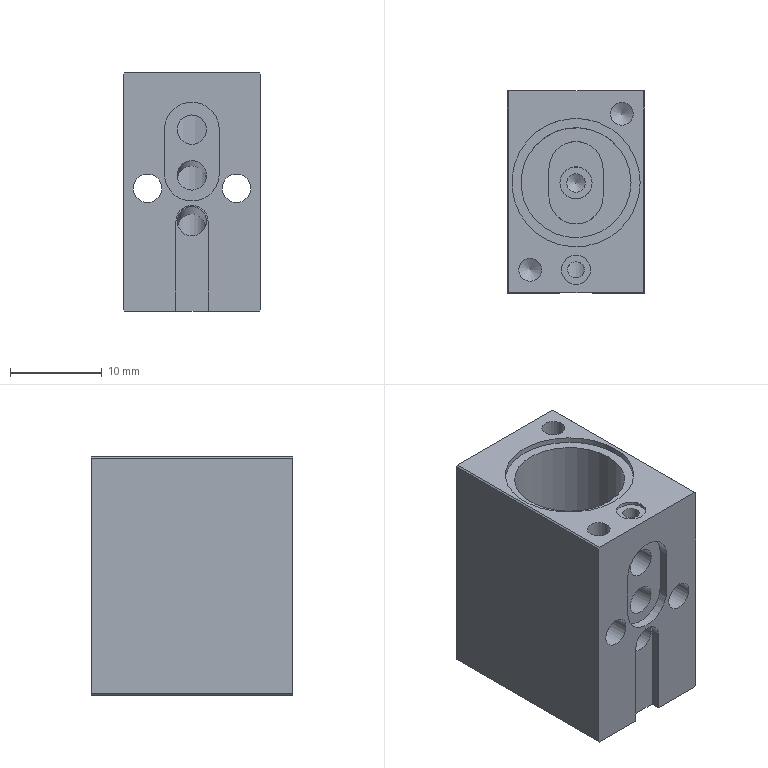NC program | NX | posted with a generic post | part box 15 x 22 x 26 mm
Lines 1 to 1765 of 5185, first 1455 of 1737 lines:
N10 G17 G21 G94 G90
(DRILLING_2 , TOOL : D4点钻)
N12 T02 M6
N14 G54
N16 G17 G0 G90 X0. Y12. B0. C0. S3000 M3
N18 G43 Z30. H2
N20 G94 G81 G98 Z-1.25 F200. R3.
N22 X5. Y19.5
N24 X0. Y2.5
N26 X-5.
N28 G80
N30 G0 X-5. Y2.5 Z30.
N32 M5
(DRILLING_2_COPY_2 , TOOL : D1.8钻头)
N34 T07 M6
N36 G54
N38 G17 G0 G90 X0. Y2.5 B0. C0. S3000 M3
N40 G43 Z30. H7
N42 G94 G81 G98 Z-6.5 F200. R3.
N44 G80
N46 G0 X0. Y2.5 Z30.
N48 M5
(DRILLING_2_COPY_1 , TOOL : D2.3钻头)
N50 T08 M6
N52 G54
N54 G17 G0 G90 X5. Y19.5 B0. C0. S3000 M3
N56 G43 Z30. H8
N58 G94 G81 G98 Z-8. F200. R3.
N60 X-5. Y2.5
N62 G80
N64 G0 X-5. Y2.5 Z30.
N66 M5
(DRILLING_2_COPY , TOOL : Z5.5)
N68 T09 M6
N70 G54
N72 G17 G0 G90 X0. Y12. B0. C0. S3000 M3
N74 G43 Z30. H9
N76 G94 G81 G99 Z-14. F200. R3.
N78 G80
N80 G0 X0. Y12. Z30.
N82 M5
(PLANAR_MILL_6 , TOOL : D8开粗)
N84 T13 M6
N86 G54
N88 G17 G0 G90 X-1.873 Y12.414 B0. C0. S4500 M3
N90 G43 Z30. H13
N92 Z1.
N94 G94 G1 X-1.9 Y11.661 Z0.987 F1000.
N96 X-1.671 Y11.035 Z0.975
N98 X-1.244 Y10.524 Z0.964
N100 X-0.656 Y10.185 Z0.952
N102 X0.17 Y10.078 Z0.937
N104 X0.965 Y10.329 Z0.923
N106 X1.58 Y10.891 Z0.908
N108 X1.9 Y11.661 Z0.893
N110 Y12.339 Z0.882
N112 X1.58 Y13.109 Z0.867
N114 X0.965 Y13.671 Z0.853
N116 X0.17 Y13.922 Z0.838
N118 X-0.656 Y13.815 Z0.823
N120 X-1.244 Y13.476 Z0.812
N122 X-1.671 Y12.965 Z0.8
N124 X-1.9 Y12.339 Z0.788
N126 Y11.661 Z0.777
N128 X-1.671 Y11.035 Z0.765
N130 X-1.244 Y10.524 Z0.753
N132 X-0.656 Y10.185 Z0.741
N134 X0.17 Y10.078 Z0.727
N136 X0.965 Y10.329 Z0.712
N138 X1.58 Y10.891 Z0.698
N140 X1.9 Y11.661 Z0.683
N142 Y12.339 Z0.671
N144 X1.58 Y13.109 Z0.657
N146 X0.965 Y13.671 Z0.642
N148 X0.17 Y13.922 Z0.628
N150 X-0.656 Y13.815 Z0.613
N152 X-1.244 Y13.476 Z0.601
N154 X-1.671 Y12.965 Z0.59
N156 X-1.9 Y12.339 Z0.578
N158 Y11.661 Z0.566
N160 X-1.671 Y11.035 Z0.555
N162 X-1.244 Y10.524 Z0.543
N164 X-0.656 Y10.185 Z0.531
N166 X0.17 Y10.078 Z0.517
N168 X0.965 Y10.329 Z0.502
N170 X1.58 Y10.891 Z0.487
N172 X1.9 Y11.661 Z0.473
N174 Y12.339 Z0.461
N176 X1.58 Y13.109 Z0.447
N178 X0.965 Y13.671 Z0.432
N180 X0.17 Y13.922 Z0.417
N182 X-0.656 Y13.815 Z0.403
N184 X-1.244 Y13.476 Z0.391
N186 X-1.671 Y12.965 Z0.379
N188 X-1.9 Y12.339 Z0.368
N190 Y11.661 Z0.356
N192 X-1.671 Y11.035 Z0.344
N194 X-1.244 Y10.524 Z0.333
N196 X-0.656 Y10.185 Z0.321
N198 X0.17 Y10.078 Z0.306
N200 X0.965 Y10.329 Z0.292
N202 X1.58 Y10.891 Z0.277
N204 X1.9 Y11.661 Z0.263
N206 Y12.339 Z0.251
N208 X1.58 Y13.109 Z0.236
N210 X0.965 Y13.671 Z0.222
N212 X0.17 Y13.922 Z0.207
N214 X-0.656 Y13.815 Z0.193
N216 X-1.244 Y13.476 Z0.181
N218 X-1.671 Y12.965 Z0.169
N220 X-1.9 Y12.339 Z0.158
N222 Y11.661 Z0.146
N224 X-1.671 Y11.035 Z0.134
N226 X-1.244 Y10.524 Z0.122
N228 X-0.656 Y10.185 Z0.111
N230 X0.17 Y10.078 Z0.096
N232 X0.965 Y10.329 Z0.082
N234 X1.58 Y10.891 Z0.067
N236 X1.9 Y11.661 Z0.052
N238 Y12.339 Z0.041
N240 X1.58 Y13.109 Z0.026
N242 X0.965 Y13.671 Z0.011
N244 X0.17 Y13.922 Z-0.003
N246 X-0.656 Y13.815 Z-0.018
N248 X-1.244 Y13.476 Z-0.029
N250 X-1.671 Y12.965 Z-0.041
N252 X-1.9 Y12.339 Z-0.053
N254 Y11.661 Z-0.065
N256 X-1.671 Y11.035 Z-0.076
N258 X-1.244 Y10.524 Z-0.088
N260 X-0.656 Y10.185 Z-0.1
N262 X0.17 Y10.078 Z-0.114
N264 X0.965 Y10.329 Z-0.129
N266 X1.58 Y10.891 Z-0.143
N268 X1.9 Y11.661 Z-0.158
N270 Y12.339 Z-0.17
N272 X1.58 Y13.109 Z-0.184
N274 X0.965 Y13.671 Z-0.199
N276 X0.17 Y13.922 Z-0.213
N278 X-0.656 Y13.815 Z-0.228
N280 X-1.244 Y13.476 Z-0.24
N282 X-1.671 Y12.965 Z-0.251
N284 X-1.9 Y12.339 Z-0.263
N286 Y11.661 Z-0.275
N288 X-1.671 Y11.035 Z-0.286
N290 X-1.244 Y10.524 Z-0.298
N292 X-0.656 Y10.185 Z-0.31
N294 X0.17 Y10.078 Z-0.324
N296 X0.965 Y10.329 Z-0.339
N298 X1.58 Y10.891 Z-0.354
N300 X1.9 Y11.661 Z-0.368
N302 Y12.339 Z-0.38
N304 X1.58 Y13.109 Z-0.394
N306 X0.965 Y13.671 Z-0.409
N308 X0.17 Y13.922 Z-0.424
N310 X-0.656 Y13.815 Z-0.438
N312 X-1.244 Y13.476 Z-0.45
N314 X-1.671 Y12.965 Z-0.462
N316 X-1.9 Y12.339 Z-0.473
N318 Y11.661 Z-0.485
N320 X-1.671 Y11.035 Z-0.497
N322 X-1.244 Y10.524 Z-0.508
N324 X-0.656 Y10.185 Z-0.52
N326 X0.17 Y10.078 Z-0.535
N328 X0.965 Y10.329 Z-0.549
N330 X1.58 Y10.891 Z-0.564
N332 X1.9 Y11.661 Z-0.578
N334 Y12.339 Z-0.59
N336 X1.58 Y13.109 Z-0.605
N338 X0.965 Y13.671 Z-0.619
N340 X0.17 Y13.922 Z-0.634
N342 X-0.656 Y13.815 Z-0.648
N344 X-1.244 Y13.476 Z-0.66
N346 X-1.671 Y12.965 Z-0.672
N348 X-1.9 Y12.339 Z-0.684
N350 Y11.661 Z-0.695
N352 X-1.671 Y11.035 Z-0.707
N354 X-1.244 Y10.524 Z-0.719
N356 X-0.656 Y10.185 Z-0.73
N358 X0.17 Y10.078 Z-0.745
N360 X0.965 Y10.329 Z-0.76
N362 X1.58 Y10.891 Z-0.774
N364 X1.9 Y11.661 Z-0.789
N366 Y12.339 Z-0.8
N368 X1.58 Y13.109 Z-0.815
N370 X0.965 Y13.671 Z-0.83
N372 X0.17 Y13.922 Z-0.844
N374 X-0.656 Y13.815 Z-0.859
N376 X-1.244 Y13.476 Z-0.871
N378 X-1.671 Y12.965 Z-0.882
N380 X-1.9 Y12.339 Z-0.894
N382 Y11.661 Z-0.906
N384 X-1.671 Y11.035 Z-0.917
N386 X-1.244 Y10.524 Z-0.929
N388 X-0.656 Y10.185 Z-0.941
N390 X0.17 Y10.078 Z-0.955
N392 X0.965 Y10.329 Z-0.97
N394 X1.58 Y10.891 Z-0.984
N396 X1.9 Y11.661 Z-0.999
N398 Y12.339 Z-1.011
N400 X1.58 Y13.109 Z-1.025
N402 X0.965 Y13.671 Z-1.04
N404 X0.17 Y13.922 Z-1.054
N406 X-0.656 Y13.815 Z-1.069
N408 X-1.244 Y13.476 Z-1.081
N410 X-1.671 Y12.965 Z-1.092
N412 X-1.9 Y12.339 Z-1.104
N414 Y11.661 Z-1.116
N416 X-1.671 Y11.035 Z-1.128
N418 X-1.244 Y10.524 Z-1.139
N420 X-0.656 Y10.185 Z-1.151
N422 X0.17 Y10.078 Z-1.166
N424 X0.965 Y10.329 Z-1.18
N426 X1.58 Y10.891 Z-1.195
N428 X1.9 Y11.661 Z-1.209
N430 Y12.339 Z-1.221
N432 X1.58 Y13.109 Z-1.236
N434 X0.965 Y13.671 Z-1.25
N436 X0.17 Y13.922 Z-1.265
N438 X-0.656 Y13.815 Z-1.279
N440 X-1.244 Y13.476 Z-1.291
N442 X-1.671 Y12.965 Z-1.303
N444 X-1.9 Y12.339 Z-1.314
N446 Y11.661 Z-1.326
N448 X-1.671 Y11.035 Z-1.338
N450 X-1.244 Y10.524 Z-1.349
N452 X-0.656 Y10.185 Z-1.361
N454 X0.17 Y10.078 Z-1.376
N456 X0.965 Y10.329 Z-1.39
N458 X1.58 Y10.891 Z-1.405
N460 X1.9 Y11.661 Z-1.419
N462 Y12.339 Z-1.431
N464 X1.58 Y13.109 Z-1.446
N466 X0.965 Y13.671 Z-1.46
N468 X0.17 Y13.922 Z-1.475
N470 X-0.656 Y13.815 Z-1.489
N472 X-1.244 Y13.476 Z-1.501
N474 X-1.671 Y12.965 Z-1.513
N476 X-1.9 Y12.339 Z-1.525
N478 Y11.661 Z-1.536
N480 X-1.671 Y11.035 Z-1.548
N482 X-1.244 Y10.524 Z-1.56
N484 X-0.656 Y10.185 Z-1.572
N486 X0.17 Y10.078 Z-1.586
N488 X0.965 Y10.329 Z-1.601
N490 X1.58 Y10.891 Z-1.615
N492 X1.9 Y11.661 Z-1.63
N494 Y12.339 Z-1.642
N496 X1.58 Y13.109 Z-1.656
N498 X0.965 Y13.671 Z-1.671
N500 X0.17 Y13.922 Z-1.685
N502 X-0.656 Y13.815 Z-1.7
N504 X-1.244 Y13.476 Z-1.712
N506 X-1.671 Y12.965 Z-1.723
N508 X-1.9 Y12.339 Z-1.735
N510 Y11.661 Z-1.747
N512 X-1.671 Y11.035 Z-1.758
N514 X-1.244 Y10.524 Z-1.77
N516 X-0.656 Y10.185 Z-1.782
N518 X0.17 Y10.078 Z-1.796
N520 X0.965 Y10.329 Z-1.811
N522 X1.58 Y10.891 Z-1.825
N524 X1.9 Y11.661 Z-1.84
N526 Y12.339 Z-1.852
N528 X1.58 Y13.109 Z-1.866
N530 X0.965 Y13.671 Z-1.881
N532 X0.17 Y13.922 Z-1.895
N534 X-0.656 Y13.815 Z-1.91
N536 X-1.244 Y13.476 Z-1.922
N538 X-1.671 Y12.965 Z-1.933
N540 X-1.9 Y12.339 Z-1.945
N542 Y11.661 Z-1.957
N544 X-1.671 Y11.035 Z-1.969
N546 X-1.244 Y10.524 Z-1.98
N548 X-0.656 Y10.185 Z-1.992
N550 X0.17 Y10.078 Z-2.007
N552 X0.965 Y10.329 Z-2.021
N554 X1.58 Y10.891 Z-2.036
N556 X1.9 Y11.661 Z-2.05
N558 Y12.339 Z-2.062
N560 X1.58 Y13.109 Z-2.077
N562 X0.965 Y13.671 Z-2.091
N564 X0.17 Y13.922 Z-2.106
N566 X-0.656 Y13.815 Z-2.12
N568 X-1.244 Y13.476 Z-2.132
N570 X-1.671 Y12.965 Z-2.144
N572 X-1.9 Y12.339 Z-2.155
N574 Y11.661 Z-2.167
N576 X-1.671 Y11.035 Z-2.179
N578 X-1.244 Y10.524 Z-2.19
N580 X-0.656 Y10.185 Z-2.202
N582 X0.17 Y10.078 Z-2.217
N584 X0.965 Y10.329 Z-2.231
N586 X1.58 Y10.891 Z-2.246
N588 X1.9 Y11.661 Z-2.26
N590 Y12.339 Z-2.272
N592 X1.58 Y13.109 Z-2.287
N594 X0.965 Y13.671 Z-2.301
N596 X0.17 Y13.922 Z-2.316
N598 X-0.656 Y13.815 Z-2.331
N600 X-1.244 Y13.476 Z-2.342
N602 X-1.671 Y12.965 Z-2.354
N604 X-1.9 Y12.339 Z-2.366
N606 Y11.661 Z-2.377
N608 X-1.671 Y11.035 Z-2.389
N610 X-1.244 Y10.524 Z-2.401
N612 X-0.656 Y10.185 Z-2.413
N614 X0.17 Y10.078 Z-2.427
N616 X0.965 Y10.329 Z-2.442
N618 X1.58 Y10.891 Z-2.456
N620 X1.9 Y11.661 Z-2.471
N622 Y12.339 Z-2.483
N624 X1.58 Y13.109 Z-2.497
N626 X0.965 Y13.671 Z-2.512
N628 X0.17 Y13.922 Z-2.526
N630 X-0.656 Y13.815 Z-2.541
N632 X-1.244 Y13.476 Z-2.553
N634 X-1.671 Y12.965 Z-2.564
N636 X-1.9 Y12.339 Z-2.576
N638 Y11.661 Z-2.588
N640 X-1.671 Y11.035 Z-2.599
N642 X-1.244 Y10.524 Z-2.611
N644 X-0.656 Y10.185 Z-2.623
N646 X0.17 Y10.078 Z-2.637
N648 X0.965 Y10.329 Z-2.652
N650 X1.58 Y10.891 Z-2.666
N652 X1.9 Y11.661 Z-2.681
N654 Y12.339 Z-2.693
N656 X1.58 Y13.109 Z-2.707
N658 X0.965 Y13.671 Z-2.722
N660 X0.17 Y13.922 Z-2.737
N662 X-0.656 Y13.815 Z-2.751
N664 X-1.244 Y13.476 Z-2.763
N666 X-1.671 Y12.965 Z-2.775
N668 X-1.9 Y12.339 Z-2.786
N670 Y11.661 Z-2.798
N672 X-1.671 Y11.035 Z-2.81
N674 X-1.244 Y10.524 Z-2.821
N676 X-0.656 Y10.185 Z-2.833
N678 X0.17 Y10.078 Z-2.848
N680 X0.965 Y10.329 Z-2.862
N682 X1.58 Y10.891 Z-2.877
N684 X1.9 Y11.661 Z-2.891
N686 Y12.339 Z-2.903
N688 X1.58 Y13.109 Z-2.918
N690 X0.965 Y13.671 Z-2.932
N692 X0.17 Y13.922 Z-2.947
N694 X-0.656 Y13.815 Z-2.961
N696 X-1.244 Y13.476 Z-2.973
N698 X-1.671 Y12.965 Z-2.985
N700 X-1.9 Y12.339 Z-2.996
N702 Y11.661 Z-3.008
N704 X-1.671 Y11.035 Z-3.02
N706 X-1.244 Y10.524 Z-3.032
N708 X-0.656 Y10.185 Z-3.043
N710 X0.17 Y10.078 Z-3.058
N712 X0.965 Y10.329 Z-3.072
N714 X1.58 Y10.891 Z-3.087
N716 X1.9 Y11.661 Z-3.102
N718 Y12.339 Z-3.113
N720 X1.58 Y13.109 Z-3.128
N722 X0.965 Y13.671 Z-3.142
N724 X0.17 Y13.922 Z-3.157
N726 X-0.656 Y13.815 Z-3.172
N728 X-1.244 Y13.476 Z-3.183
N730 X-1.671 Y12.965 Z-3.195
N732 X-1.9 Y12.339 Z-3.207
N734 Y11.661 Z-3.219
N736 X-1.671 Y11.035 Z-3.23
N738 X-1.244 Y10.524 Z-3.242
N740 X-0.656 Y10.185 Z-3.254
N742 X0.17 Y10.078 Z-3.268
N744 X0.965 Y10.329 Z-3.283
N746 X1.58 Y10.891 Z-3.297
N748 X1.9 Y11.661 Z-3.312
N750 Y12.339 Z-3.324
N752 X1.58 Y13.109 Z-3.338
N754 X0.965 Y13.671 Z-3.353
N756 X0.17 Y13.922 Z-3.367
N758 X-0.656 Y13.815 Z-3.382
N760 X-1.244 Y13.476 Z-3.394
N762 X-1.671 Y12.965 Z-3.405
N764 X-1.9 Y12.339 Z-3.417
N766 Y11.661 Z-3.429
N768 X-1.671 Y11.035 Z-3.44
N770 X-1.244 Y10.524 Z-3.452
N772 X-0.656 Y10.185 Z-3.464
N774 X0.17 Y10.078 Z-3.478
N776 X0.965 Y10.329 Z-3.493
N778 X1.58 Y10.891 Z-3.508
N780 X1.9 Y11.661 Z-3.522
N782 Y12.339 Z-3.534
N784 X1.58 Y13.109 Z-3.548
N786 X0.965 Y13.671 Z-3.563
N788 X0.17 Y13.922 Z-3.578
N790 X-0.656 Y13.815 Z-3.592
N792 X-1.244 Y13.476 Z-3.604
N794 X-1.671 Y12.965 Z-3.616
N796 X-1.9 Y12.339 Z-3.627
N798 Y11.661 Z-3.639
N800 X-1.671 Y11.035 Z-3.651
N802 X-1.244 Y10.524 Z-3.662
N804 X-0.656 Y10.185 Z-3.674
N806 X0.17 Y10.078 Z-3.689
N808 X0.965 Y10.329 Z-3.703
N810 X1.58 Y10.891 Z-3.718
N812 X1.9 Y11.661 Z-3.732
N814 Y12.339 Z-3.744
N816 X1.58 Y13.109 Z-3.759
N818 X0.965 Y13.671 Z-3.773
N820 X0.17 Y13.922 Z-3.788
N822 X-0.656 Y13.815 Z-3.802
N824 X-1.244 Y13.476 Z-3.814
N826 X-1.671 Y12.965 Z-3.826
N828 X-1.9 Y12.339 Z-3.837
N830 Y11.661 Z-3.849
N832 X-1.671 Y11.035 Z-3.861
N834 X-1.244 Y10.524 Z-3.873
N836 X-0.656 Y10.185 Z-3.884
N838 X0.17 Y10.078 Z-3.899
N840 X0.965 Y10.329 Z-3.914
N842 X1.58 Y10.891 Z-3.928
N844 X1.9 Y11.661 Z-3.943
N846 Y12.339 Z-3.954
N848 X1.58 Y13.109 Z-3.969
N850 X0.965 Y13.671 Z-3.984
N852 X0.17 Y13.922 Z-3.998
N854 X-0.656 Y13.815 Z-4.013
N856 X-1.244 Y13.476 Z-4.024
N858 X-1.671 Y12.965 Z-4.036
N860 X-1.9 Y12.339 Z-4.048
N862 Y11.661 Z-4.06
N864 X-1.671 Y11.035 Z-4.071
N866 X-1.244 Y10.524 Z-4.083
N868 X-0.656 Y10.185 Z-4.095
N870 X0.17 Y10.078 Z-4.109
N872 X0.965 Y10.329 Z-4.124
N874 X1.58 Y10.891 Z-4.138
N876 X1.9 Y11.661 Z-4.153
N878 Y12.339 Z-4.165
N880 X1.58 Y13.109 Z-4.179
N882 X0.965 Y13.671 Z-4.194
N884 X0.17 Y13.922 Z-4.208
N886 X-0.656 Y13.815 Z-4.223
N888 X-1.244 Y13.476 Z-4.235
N890 X-1.671 Y12.965 Z-4.246
N892 X-1.9 Y12.339 Z-4.258
N894 Y11.661 Z-4.27
N896 X-1.671 Y11.035 Z-4.281
N898 X-1.244 Y10.524 Z-4.293
N900 X-0.656 Y10.185 Z-4.305
N902 X0.17 Y10.078 Z-4.319
N904 X0.965 Y10.329 Z-4.334
N906 X1.58 Y10.891 Z-4.349
N908 X1.9 Y11.661 Z-4.363
N910 Y12.339 Z-4.375
N912 X1.58 Y13.109 Z-4.39
N914 X0.965 Y13.671 Z-4.404
N916 X0.17 Y13.922 Z-4.419
N918 X-0.656 Y13.815 Z-4.433
N920 X-1.244 Y13.476 Z-4.445
N922 X-1.671 Y12.965 Z-4.457
N924 X-1.9 Y12.339 Z-4.468
N926 Y11.661 Z-4.48
N928 X-1.671 Y11.035 Z-4.492
N930 X-1.244 Y10.524 Z-4.503
N932 X-0.656 Y10.185 Z-4.515
N934 X0.17 Y10.078 Z-4.53
N936 X0.965 Y10.329 Z-4.544
N938 X1.58 Y10.891 Z-4.559
N940 X1.9 Y11.661 Z-4.573
N942 Y12.339 Z-4.585
N944 X1.58 Y13.109 Z-4.6
N946 X0.965 Y13.671 Z-4.614
N948 X0.17 Y13.922 Z-4.629
N950 X-0.656 Y13.815 Z-4.643
N952 X-1.244 Y13.476 Z-4.655
N954 X-1.671 Y12.965 Z-4.667
N956 X-1.9 Y12.339 Z-4.679
N958 Y11.661 Z-4.69
N960 X-1.671 Y11.035 Z-4.702
N962 X-1.244 Y10.524 Z-4.714
N964 X-0.656 Y10.185 Z-4.725
N966 X0.17 Y10.078 Z-4.74
N968 X0.965 Y10.329 Z-4.755
N970 X1.58 Y10.891 Z-4.769
N972 X1.9 Y11.661 Z-4.784
N974 Y12.339 Z-4.795
N976 X1.58 Y13.109 Z-4.81
N978 X0.965 Y13.671 Z-4.825
N980 X0.17 Y13.922 Z-4.839
N982 X-0.656 Y13.815 Z-4.854
N984 X-1.244 Y13.476 Z-4.866
N986 X-1.671 Y12.965 Z-4.877
N988 X-1.9 Y12.339 Z-4.889
N990 Y11.661 Z-4.901
N992 X-1.671 Y11.035 Z-4.912
N994 X-1.244 Y10.524 Z-4.924
N996 X-0.656 Y10.185 Z-4.936
N998 X0.17 Y10.078 Z-4.95
N1000 X0.965 Y10.329 Z-4.965
N1002 X1.58 Y10.891 Z-4.979
N1004 X1.9 Y11.661 Z-4.994
N1006 Y12.339 Z-5.006
N1008 X1.58 Y13.109 Z-5.02
N1010 X0.965 Y13.671 Z-5.035
N1012 X0.17 Y13.922 Z-5.049
N1014 X-0.656 Y13.815 Z-5.064
N1016 X-1.244 Y13.476 Z-5.076
N1018 X-1.671 Y12.965 Z-5.087
N1020 X-1.9 Y12.339 Z-5.099
N1022 Y11.661 Z-5.111
N1024 X-1.671 Y11.035 Z-5.123
N1026 X-1.244 Y10.524 Z-5.134
N1028 X-0.656 Y10.185 Z-5.146
N1030 X0.17 Y10.078 Z-5.161
N1032 X0.965 Y10.329 Z-5.175
N1034 X1.58 Y10.891 Z-5.19
N1036 X1.9 Y11.661 Z-5.204
N1038 Y12.339 Z-5.216
N1040 X1.58 Y13.109 Z-5.231
N1042 X0.965 Y13.671 Z-5.245
N1044 X0.17 Y13.922 Z-5.26
N1046 X-0.656 Y13.815 Z-5.274
N1048 X-1.244 Y13.476 Z-5.286
N1050 X-1.671 Y12.965 Z-5.298
N1052 X-1.9 Y12.339 Z-5.309
N1054 Y11.661 Z-5.321
N1056 X-1.671 Y11.035 Z-5.333
N1058 X-1.244 Y10.524 Z-5.344
N1060 X-0.656 Y10.185 Z-5.356
N1062 X0.17 Y10.078 Z-5.371
N1064 X0.965 Y10.329 Z-5.385
N1066 X1.58 Y10.891 Z-5.4
N1068 X1.9 Y11.661 Z-5.414
N1070 Y12.339 Z-5.426
N1072 X1.58 Y13.109 Z-5.441
N1074 X0.965 Y13.671 Z-5.455
N1076 X0.17 Y13.922 Z-5.47
N1078 X-0.656 Y13.815 Z-5.484
N1080 X-1.244 Y13.476 Z-5.496
N1082 X-1.671 Y12.965 Z-5.508
N1084 X-1.9 Y12.339 Z-5.52
N1086 Y11.661 Z-5.531
N1088 X-1.671 Y11.035 Z-5.543
N1090 X-1.244 Y10.524 Z-5.555
N1092 X-0.656 Y10.185 Z-5.567
N1094 X0.17 Y10.078 Z-5.581
N1096 X0.965 Y10.329 Z-5.596
N1098 X1.58 Y10.891 Z-5.61
N1100 X1.9 Y11.661 Z-5.625
N1102 Y12.339 Z-5.637
N1104 X1.58 Y13.109 Z-5.651
N1106 X0.965 Y13.671 Z-5.666
N1108 X0.17 Y13.922 Z-5.68
N1110 X-0.656 Y13.815 Z-5.695
N1112 X-1.244 Y13.476 Z-5.707
N1114 X-1.671 Y12.965 Z-5.718
N1116 X-1.9 Y12.339 Z-5.73
N1118 Y11.661 Z-5.742
N1120 X-1.671 Y11.035 Z-5.753
N1122 X-1.244 Y10.524 Z-5.765
N1124 X-0.656 Y10.185 Z-5.777
N1126 X0.17 Y10.078 Z-5.791
N1128 X0.965 Y10.329 Z-5.806
N1130 X1.58 Y10.891 Z-5.82
N1132 X1.9 Y11.661 Z-5.835
N1134 Y12.339 Z-5.847
N1136 X1.58 Y13.109 Z-5.861
N1138 X0.965 Y13.671 Z-5.876
N1140 X0.17 Y13.922 Z-5.89
N1142 X-0.656 Y13.815 Z-5.905
N1144 X-1.244 Y13.476 Z-5.917
N1146 X-1.671 Y12.965 Z-5.928
N1148 X-1.9 Y12.339 Z-5.94
N1150 Y11.661 Z-5.952
N1152 X-1.671 Y11.035 Z-5.964
N1154 X-1.244 Y10.524 Z-5.975
N1156 X-0.656 Y10.185 Z-5.987
N1158 X0.17 Y10.078 Z-6.002
N1160 X0.965 Y10.329 Z-6.016
N1162 X1.58 Y10.891 Z-6.031
N1164 X1.9 Y11.661 Z-6.045
N1166 Y12.339 Z-6.057
N1168 X1.58 Y13.109 Z-6.072
N1170 X0.965 Y13.671 Z-6.086
N1172 X0.17 Y13.922 Z-6.101
N1174 X-0.656 Y13.815 Z-6.115
N1176 X-1.244 Y13.476 Z-6.127
N1178 X-1.671 Y12.965 Z-6.139
N1180 X-1.9 Y12.339 Z-6.15
N1182 Y11.661 Z-6.162
N1184 X-1.671 Y11.035 Z-6.174
N1186 X-1.244 Y10.524 Z-6.185
N1188 X-0.656 Y10.185 Z-6.197
N1190 X0.17 Y10.078 Z-6.212
N1192 X0.965 Y10.329 Z-6.226
N1194 X1.58 Y10.891 Z-6.241
N1196 X1.9 Y11.661 Z-6.256
N1198 Y12.339 Z-6.267
N1200 X1.58 Y13.109 Z-6.282
N1202 X0.965 Y13.671 Z-6.296
N1204 X0.17 Y13.922 Z-6.311
N1206 X-0.656 Y13.815 Z-6.326
N1208 X-1.244 Y13.476 Z-6.337
N1210 X-1.671 Y12.965 Z-6.349
N1212 X-1.9 Y12.339 Z-6.361
N1214 Y11.661 Z-6.372
N1216 X-1.671 Y11.035 Z-6.384
N1218 X-1.244 Y10.524 Z-6.396
N1220 X-0.656 Y10.185 Z-6.408
N1222 X0.17 Y10.078 Z-6.422
N1224 X0.965 Y10.329 Z-6.437
N1226 X1.58 Y10.891 Z-6.451
N1228 X1.9 Y11.661 Z-6.466
N1230 Y12.339 Z-6.478
N1232 X1.58 Y13.109 Z-6.492
N1234 X0.965 Y13.671 Z-6.507
N1236 X0.17 Y13.922 Z-6.521
N1238 X-0.656 Y13.815 Z-6.536
N1240 X-1.244 Y13.476 Z-6.548
N1242 X-1.671 Y12.965 Z-6.559
N1244 X-1.9 Y12.339 Z-6.571
N1246 Y11.661 Z-6.583
N1248 X-1.671 Y11.035 Z-6.594
N1250 X-1.244 Y10.524 Z-6.606
N1252 X-0.656 Y10.185 Z-6.618
N1254 X0.17 Y10.078 Z-6.632
N1256 X0.965 Y10.329 Z-6.647
N1258 X1.58 Y10.891 Z-6.661
N1260 X1.9 Y11.661 Z-6.676
N1262 Y12.339 Z-6.688
N1264 X1.58 Y13.109 Z-6.702
N1266 X0.965 Y13.671 Z-6.717
N1268 X0.17 Y13.922 Z-6.732
N1270 X-0.656 Y13.815 Z-6.746
N1272 X-1.244 Y13.476 Z-6.758
N1274 X-1.671 Y12.965 Z-6.77
N1276 X-1.9 Y12.339 Z-6.781
N1278 Y11.661 Z-6.793
N1280 X-1.671 Y11.035 Z-6.805
N1282 X-1.244 Y10.524 Z-6.816
N1284 X-0.656 Y10.185 Z-6.828
N1286 X0.17 Y10.078 Z-6.843
N1288 X0.965 Y10.329 Z-6.857
N1290 X1.58 Y10.891 Z-6.872
N1292 X1.9 Y11.661 Z-6.886
N1294 Y12.339 Z-6.898
N1296 X1.58 Y13.109 Z-6.913
N1298 X0.965 Y13.671 Z-6.927
N1300 X0.17 Y13.922 Z-6.942
N1302 X-0.656 Y13.815 Z-6.956
N1304 X-1.244 Y13.476 Z-6.968
N1306 X-1.671 Y12.965 Z-6.98
N1308 X-1.9 Y12.339 Z-6.991
N1310 Y11.661 Z-7.003
N1312 X-1.671 Y11.035 Z-7.015
N1314 X-1.244 Y10.524 Z-7.027
N1316 X-0.656 Y10.185 Z-7.038
N1318 X0.17 Y10.078 Z-7.053
N1320 X0.965 Y10.329 Z-7.067
N1322 X1.58 Y10.891 Z-7.082
N1324 X1.9 Y11.661 Z-7.097
N1326 Y12.339 Z-7.108
N1328 X1.58 Y13.109 Z-7.123
N1330 X0.965 Y13.671 Z-7.138
N1332 X0.17 Y13.922 Z-7.152
N1334 X-0.656 Y13.815 Z-7.167
N1336 X-1.244 Y13.476 Z-7.178
N1338 X-1.671 Y12.965 Z-7.19
N1340 X-1.9 Y12.339 Z-7.202
N1342 Y11.661 Z-7.214
N1344 X-1.671 Y11.035 Z-7.225
N1346 X-1.244 Y10.524 Z-7.237
N1348 X-0.656 Y10.185 Z-7.249
N1350 X0.17 Y10.078 Z-7.263
N1352 X0.965 Y10.329 Z-7.278
N1354 X1.58 Y10.891 Z-7.292
N1356 X1.9 Y11.661 Z-7.307
N1358 Y12.339 Z-7.319
N1360 X1.58 Y13.109 Z-7.333
N1362 X0.965 Y13.671 Z-7.348
N1364 X0.17 Y13.922 Z-7.362
N1366 X-0.656 Y13.815 Z-7.377
N1368 X-1.244 Y13.476 Z-7.389
N1370 X-1.671 Y12.965 Z-7.4
N1372 X-1.9 Y12.339 Z-7.412
N1374 Y11.661 Z-7.424
N1376 X-1.671 Y11.035 Z-7.435
N1378 X-1.244 Y10.524 Z-7.447
N1380 X-0.656 Y10.185 Z-7.459
N1382 X0.17 Y10.078 Z-7.473
N1384 X0.965 Y10.329 Z-7.488
N1386 X1.58 Y10.891 Z-7.503
N1388 X1.9 Y11.661 Z-7.517
N1390 Y12.339 Z-7.529
N1392 X1.58 Y13.109 Z-7.543
N1394 X0.965 Y13.671 Z-7.558
N1396 X0.17 Y13.922 Z-7.573
N1398 X-0.656 Y13.815 Z-7.587
N1400 X-1.244 Y13.476 Z-7.599
N1402 X-1.671 Y12.965 Z-7.611
N1404 X-1.9 Y12.339 Z-7.622
N1406 Y11.661 Z-7.634
N1408 X-1.671 Y11.035 Z-7.646
N1410 X-1.244 Y10.524 Z-7.657
N1412 X-0.656 Y10.185 Z-7.669
N1414 X0.17 Y10.078 Z-7.684
N1416 X0.965 Y10.329 Z-7.698
N1418 X1.58 Y10.891 Z-7.713
N1420 X1.9 Y11.661 Z-7.727
N1422 Y12.339 Z-7.739
N1424 X1.58 Y13.109 Z-7.754
N1426 X0.965 Y13.671 Z-7.768
N1428 X0.17 Y13.922 Z-7.783
N1430 X-0.656 Y13.815 Z-7.797
N1432 X-1.244 Y13.476 Z-7.809
N1434 X-1.671 Y12.965 Z-7.821
N1436 X-1.9 Y12.339 Z-7.832
N1438 Y11.661 Z-7.844
N1440 X-1.671 Y11.035 Z-7.856
N1442 X-1.244 Y10.524 Z-7.868
N1444 X-0.656 Y10.185 Z-7.879
N1446 X0.17 Y10.078 Z-7.894
N1448 X0.965 Y10.329 Z-7.909
N1450 X1.58 Y10.891 Z-7.923
N1452 X1.9 Y11.661 Z-7.938
N1454 Y12.339 Z-7.949
N1456 X1.58 Y13.109 Z-7.964
N1458 X0.965 Y13.671 Z-7.979
N1460 X0.17 Y13.922 Z-7.993
N1462 X-0.656 Y13.815 Z-8.008
N1464 X-1.244 Y13.476 Z-8.019
N1466 X-1.671 Y12.965 Z-8.031
N1468 X-1.9 Y12.339 Z-8.043
N1470 Y11.661 Z-8.055
N1472 X-1.671 Y11.035 Z-8.066
N1474 X-1.244 Y10.524 Z-8.078
N1476 X-0.656 Y10.185 Z-8.09
N1478 X0.17 Y10.078 Z-8.104
N1480 X0.965 Y10.329 Z-8.119
N1482 X1.58 Y10.891 Z-8.133
N1484 X1.9 Y11.661 Z-8.148
N1486 Y12.339 Z-8.16
N1488 X1.58 Y13.109 Z-8.174
N1490 X0.965 Y13.671 Z-8.189
N1492 X0.17 Y13.922 Z-8.203
N1494 X-0.656 Y13.815 Z-8.218
N1496 X-1.244 Y13.476 Z-8.23
N1498 X-1.671 Y12.965 Z-8.241
N1500 X-1.9 Y12.339 Z-8.253
N1502 Y11.661 Z-8.265
N1504 X-1.671 Y11.035 Z-8.276
N1506 X-1.244 Y10.524 Z-8.288
N1508 X-0.656 Y10.185 Z-8.3
N1510 X0.17 Y10.078 Z-8.315
N1512 X0.965 Y10.329 Z-8.329
N1514 X1.58 Y10.891 Z-8.344
N1516 X1.9 Y11.661 Z-8.358
N1518 Y12.339 Z-8.37
N1520 X1.58 Y13.109 Z-8.385
N1522 X0.965 Y13.671 Z-8.399
N1524 X0.17 Y13.922 Z-8.414
N1526 X-0.656 Y13.815 Z-8.428
N1528 X-1.244 Y13.476 Z-8.44
N1530 X-1.671 Y12.965 Z-8.452
N1532 X-1.9 Y12.339 Z-8.463
N1534 Y11.661 Z-8.475
N1536 X-1.671 Y11.035 Z-8.487
N1538 X-1.244 Y10.524 Z-8.498
N1540 X-0.656 Y10.185 Z-8.51
N1542 X0.17 Y10.078 Z-8.525
N1544 X0.965 Y10.329 Z-8.539
N1546 X1.58 Y10.891 Z-8.554
N1548 X1.9 Y11.661 Z-8.568
N1550 Y12.339 Z-8.58
N1552 X1.58 Y13.109 Z-8.595
N1554 X0.965 Y13.671 Z-8.609
N1556 X0.17 Y13.922 Z-8.624
N1558 X-0.656 Y13.815 Z-8.638
N1560 X-1.244 Y13.476 Z-8.65
N1562 X-1.671 Y12.965 Z-8.662
N1564 X-1.9 Y12.339 Z-8.674
N1566 Y11.661 Z-8.685
N1568 X-1.671 Y11.035 Z-8.697
N1570 X-1.244 Y10.524 Z-8.709
N1572 X-0.656 Y10.185 Z-8.72
N1574 X0.17 Y10.078 Z-8.735
N1576 X0.965 Y10.329 Z-8.75
N1578 X1.58 Y10.891 Z-8.764
N1580 X1.9 Y11.661 Z-8.779
N1582 Y12.339 Z-8.791
N1584 X1.58 Y13.109 Z-8.805
N1586 X0.965 Y13.671 Z-8.82
N1588 X0.17 Y13.922 Z-8.834
N1590 X-0.656 Y13.815 Z-8.849
N1592 X-1.244 Y13.476 Z-8.861
N1594 X-1.671 Y12.965 Z-8.872
N1596 X-1.9 Y12.339 Z-8.884
N1598 Y11.661 Z-8.896
N1600 X-1.671 Y11.035 Z-8.907
N1602 X-1.244 Y10.524 Z-8.919
N1604 X-0.656 Y10.185 Z-8.931
N1606 X0.17 Y10.078 Z-8.945
N1608 X0.965 Y10.329 Z-8.96
N1610 X1.58 Y10.891 Z-8.974
N1612 X1.9 Y11.661 Z-8.989
N1614 Y12.339 Z-9.001
N1616 X1.58 Y13.109 Z-9.015
N1618 X0.965 Y13.671 Z-9.03
N1620 X0.17 Y13.922 Z-9.044
N1622 X-0.656 Y13.815 Z-9.059
N1624 X-1.244 Y13.476 Z-9.071
N1626 X-1.671 Y12.965 Z-9.082
N1628 X-1.9 Y12.339 Z-9.094
N1630 Y12. Z-9.1
N1632 G3 X0. Y10.1 R1.9
N1634 X-1.9 Y12. R-1.9
N1636 G1 Z-8.1
N1638 G0 Z30.
(PLANAR_MILL_8 , TOOL : D8开粗)
N1640 X-0.369 Y12.821
N1642 Z1.5
N1644 G1 Z-0.5 F600.
N1646 X-0.9 Y14.
N1648 G3 X-2.9 Y12. R2.
N1650 X0. Y9.1 R2.9
N1652 X-2.9 Y12. R-2.9
N1654 X-0.9 Y10. R2.
N1656 G1 X-0.369 Y11.179
N1658 Z1.5
N1660 G0 Z30.
N1662 M5
(PLANAR_MILL_7 , TOOL : D3开粗)
N1664 T14 M6
N1666 G54
N1668 G17 G0 G90 X1.276 Y9.987 B0. C0. S5500 M3
N1670 G43 Z30. H14
N1672 Z-7.2
N1674 G94 G1 X1.37 Y10.162 Z-7.202 F600.
N1676 Y13.838 Z-7.234
N1678 X0.99 Y14.54 Z-7.241
N1680 X0.288 Y14.92 Z-7.248
N1682 X-0.288 Z-7.253
N1684 X-0.99 Y14.54 Z-7.26
N1686 X-1.37 Y13.838 Z-7.267
N1688 Y10.162 Z-7.299
N1690 X-0.99 Y9.46 Z-7.306
N1692 X-0.288 Y9.08 Z-7.313
N1694 X0.288 Z-7.318
N1696 X0.99 Y9.46 Z-7.325
N1698 X1.37 Y10.162 Z-7.332
N1700 Y13.838 Z-7.364
N1702 X0.99 Y14.54 Z-7.371
N1704 X0.288 Y14.92 Z-7.378
N1706 X-0.288 Z-7.383
N1708 X-0.99 Y14.54 Z-7.39
N1710 X-1.37 Y13.838 Z-7.397
N1712 Y10.162 Z-7.429
N1714 X-0.99 Y9.46 Z-7.436
N1716 X-0.288 Y9.08 Z-7.443
N1718 X0.288 Z-7.448
N1720 X0.99 Y9.46 Z-7.455
N1722 X1.37 Y10.162 Z-7.462
N1724 Y13.838 Z-7.494
N1726 X0.99 Y14.54 Z-7.501
N1728 X0.288 Y14.92 Z-7.508
N1730 X-0.288 Z-7.513
N1732 X-0.99 Y14.54 Z-7.52
N1734 X-1.37 Y13.838 Z-7.527
N1736 Y10.162 Z-7.559
N1738 X-0.99 Y9.46 Z-7.566
N1740 X-0.288 Y9.08 Z-7.573
N1742 X0.288 Z-7.578
N1744 X0.99 Y9.46 Z-7.585
N1746 X1.37 Y10.162 Z-7.592
N1748 Y13.838 Z-7.624
N1750 X0.99 Y14.54 Z-7.631
N1752 X0.288 Y14.92 Z-7.638
N1754 X-0.288 Z-7.643
N1756 X-0.99 Y14.54 Z-7.65
N1758 X-1.37 Y13.838 Z-7.657
N1760 Y10.162 Z-7.689
N1762 X-0.99 Y9.46 Z-7.696
N1764 X-0.288 Y9.08 Z-7.703
N1766 X0.288 Z-7.708
N1768 X0.99 Y9.46 Z-7.715
N1770 X1.37 Y10.162 Z-7.722
N1772 Y13.838 Z-7.754
N1774 X0.99 Y14.54 Z-7.761
N1776 X0.288 Y14.92 Z-7.768
N1778 X-0.288 Z-7.773
N1780 X-0.99 Y14.54 Z-7.78
N1782 X-1.37 Y13.838 Z-7.786
N1784 Y10.162 Z-7.819
N1786 X-0.99 Y9.46 Z-7.826
N1788 X-0.288 Y9.08 Z-7.832
N1790 X0.288 Z-7.838
N1792 X0.99 Y9.46 Z-7.844
N1794 X1.37 Y10.162 Z-7.851
N1796 Y13.838 Z-7.884
N1798 X0.99 Y14.54 Z-7.891
N1800 X0.288 Y14.92 Z-7.897
N1802 X-0.288 Z-7.902
N1804 X-0.99 Y14.54 Z-7.909
N1806 X-1.37 Y13.838 Z-7.916
N1808 Y10.162 Z-7.949
N1810 X-0.99 Y9.46 Z-7.955
N1812 X-0.288 Y9.08 Z-7.962
N1814 X0.288 Z-7.967
N1816 X0.99 Y9.46 Z-7.974
N1818 X1.37 Y10.162 Z-7.981
N1820 Y13.838 Z-8.013
N1822 X0.99 Y14.54 Z-8.02
N1824 X0.288 Y14.92 Z-8.027
N1826 X-0.288 Z-8.032
N1828 X-0.99 Y14.54 Z-8.039
N1830 X-1.37 Y13.838 Z-8.046
N1832 Y10.162 Z-8.078
N1834 X-0.99 Y9.46 Z-8.085
N1836 X-0.288 Y9.08 Z-8.092
N1838 X0.288 Z-8.097
N1840 X0.99 Y9.46 Z-8.104
N1842 X1.37 Y10.162 Z-8.111
N1844 Y13.838 Z-8.143
N1846 X0.99 Y14.54 Z-8.15
N1848 X0.288 Y14.92 Z-8.157
N1850 X-0.288 Z-8.162
N1852 X-0.99 Y14.54 Z-8.169
N1854 X-1.37 Y13.838 Z-8.176
N1856 Y10.162 Z-8.208
N1858 X-0.99 Y9.46 Z-8.215
N1860 X-0.288 Y9.08 Z-8.222
N1862 X0.288 Z-8.227
N1864 X0.99 Y9.46 Z-8.234
N1866 X1.37 Y10.162 Z-8.241
N1868 Y13.838 Z-8.273
N1870 X0.99 Y14.54 Z-8.28
N1872 X0.288 Y14.92 Z-8.287
N1874 X-0.288 Z-8.292
N1876 X-0.99 Y14.54 Z-8.299
N1878 X-1.37 Y13.838 Z-8.306
N1880 Y10.162 Z-8.338
N1882 X-0.99 Y9.46 Z-8.345
N1884 X-0.288 Y9.08 Z-8.352
N1886 X0.288 Z-8.357
N1888 X0.99 Y9.46 Z-8.364
N1890 X1.37 Y10.162 Z-8.371
N1892 Y13.838 Z-8.403
N1894 X0.99 Y14.54 Z-8.41
N1896 X0.288 Y14.92 Z-8.417
N1898 X-0.288 Z-8.422
N1900 X-0.99 Y14.54 Z-8.429
N1902 X-1.37 Y13.838 Z-8.436
N1904 Y10.162 Z-8.468
N1906 X-0.99 Y9.46 Z-8.475
N1908 X-0.288 Y9.08 Z-8.482
N1910 X0.288 Z-8.487
N1912 X0.99 Y9.46 Z-8.494
N1914 X1.37 Y10.162 Z-8.501
N1916 Y13.838 Z-8.533
N1918 X0.99 Y14.54 Z-8.54
N1920 X0.288 Y14.92 Z-8.547
N1922 X-0.288 Z-8.552
N1924 X-0.99 Y14.54 Z-8.559
N1926 X-1.37 Y13.838 Z-8.566
N1928 Y10.162 Z-8.598
N1930 X-0.99 Y9.46 Z-8.605
N1932 X-0.288 Y9.08 Z-8.612
N1934 X0.288 Z-8.617
N1936 X0.99 Y9.46 Z-8.624
N1938 X1.37 Y10.162 Z-8.631
N1940 Y13.838 Z-8.663
N1942 X0.99 Y14.54 Z-8.67
N1944 X0.288 Y14.92 Z-8.677
N1946 X-0.288 Z-8.682
N1948 X-0.99 Y14.54 Z-8.689
N1950 X-1.37 Y13.838 Z-8.696
N1952 Y10.162 Z-8.728
N1954 X-0.99 Y9.46 Z-8.735
N1956 X-0.288 Y9.08 Z-8.742
N1958 X0.288 Z-8.747
N1960 X0.99 Y9.46 Z-8.754
N1962 X1.37 Y10.162 Z-8.761
N1964 Y13.838 Z-8.793
N1966 X0.99 Y14.54 Z-8.8
N1968 X0.288 Y14.92 Z-8.807
N1970 X-0.288 Z-8.812
N1972 X-0.99 Y14.54 Z-8.819
N1974 X-1.37 Y13.838 Z-8.826
N1976 Y10.162 Z-8.858
N1978 X-0.99 Y9.46 Z-8.865
N1980 X-0.288 Y9.08 Z-8.872
N1982 X0.288 Z-8.877
N1984 X0.99 Y9.46 Z-8.884
N1986 X1.37 Y10.162 Z-8.891
N1988 Y13.838 Z-8.923
N1990 X0.99 Y14.54 Z-8.93
N1992 X0.288 Y14.92 Z-8.937
N1994 X-0.288 Z-8.942
N1996 X-0.99 Y14.54 Z-8.949
N1998 X-1.37 Y13.838 Z-8.956
N2000 Y10.162 Z-8.988
N2002 X-0.99 Y9.46 Z-8.995
N2004 X-0.288 Y9.08 Z-9.002
N2006 X0.288 Z-9.007
N2008 X0.99 Y9.46 Z-9.014
N2010 X1.37 Y10.162 Z-9.021
N2012 Y13.838 Z-9.053
N2014 X0.99 Y14.54 Z-9.06
N2016 X0.288 Y14.92 Z-9.067
N2018 X-0.288 Z-9.072
N2020 X-0.99 Y14.54 Z-9.079
N2022 X-1.37 Y13.838 Z-9.086
N2024 Y10.162 Z-9.118
N2026 X-0.99 Y9.46 Z-9.125
N2028 X-0.288 Y9.08 Z-9.132
N2030 X0.288 Z-9.137
N2032 X0.99 Y9.46 Z-9.144
N2034 X1.37 Y10.162 Z-9.151
N2036 Y13.838 Z-9.183
N2038 X0.99 Y14.54 Z-9.19
N2040 X0.288 Y14.92 Z-9.197
N2042 X-0.288 Z-9.202
N2044 X-0.99 Y14.54 Z-9.209
N2046 X-1.37 Y13.838 Z-9.216
N2048 Y10.162 Z-9.248
N2050 X-0.99 Y9.46 Z-9.255
N2052 X-0.288 Y9.08 Z-9.262
N2054 X0.288 Z-9.267
N2056 X0.99 Y9.46 Z-9.274
N2058 X1.37 Y10.162 Z-9.281
N2060 Y13.838 Z-9.313
N2062 X0.99 Y14.54 Z-9.32
N2064 X0.288 Y14.92 Z-9.327
N2066 X-0.288 Z-9.332
N2068 X-0.99 Y14.54 Z-9.339
N2070 X-1.37 Y13.838 Z-9.346
N2072 Y10.162 Z-9.378
N2074 X-0.99 Y9.46 Z-9.385
N2076 X-0.288 Y9.08 Z-9.392
N2078 X0.288 Z-9.397
N2080 X0.99 Y9.46 Z-9.404
N2082 X1.37 Y10.162 Z-9.411
N2084 Y13.838 Z-9.443
N2086 X0.99 Y14.54 Z-9.45
N2088 X0.288 Y14.92 Z-9.457
N2090 X-0.288 Z-9.462
N2092 X-0.99 Y14.54 Z-9.469
N2094 X-1.37 Y13.838 Z-9.476
N2096 Y10.162 Z-9.508
N2098 X-0.99 Y9.46 Z-9.515
N2100 X-0.288 Y9.08 Z-9.522
N2102 X0.288 Z-9.527
N2104 X0.99 Y9.46 Z-9.534
N2106 X1.37 Y10.162 Z-9.541
N2108 Y13.838 Z-9.573
N2110 X0.99 Y14.54 Z-9.58
N2112 X0.288 Y14.92 Z-9.587
N2114 X-0.288 Z-9.592
N2116 X-0.99 Y14.54 Z-9.599
N2118 X-1.37 Y13.838 Z-9.606
N2120 Y10.162 Z-9.638
N2122 X-0.99 Y9.46 Z-9.645
N2124 X-0.288 Y9.08 Z-9.652
N2126 X0.288 Z-9.657
N2128 X0.99 Y9.46 Z-9.664
N2130 X1.37 Y10.162 Z-9.671
N2132 Y13.838 Z-9.703
N2134 X0.99 Y14.54 Z-9.71
N2136 X0.288 Y14.92 Z-9.717
N2138 X-0.288 Z-9.722
N2140 X-0.99 Y14.54 Z-9.729
N2142 X-1.37 Y13.838 Z-9.736
N2144 Y10.162 Z-9.768
N2146 X-0.99 Y9.46 Z-9.775
N2148 X-0.288 Y9.08 Z-9.782
N2150 X0.288 Z-9.787
N2152 X0.99 Y9.46 Z-9.794
N2154 X1.37 Y10.162 Z-9.801
N2156 Y13.838 Z-9.833
N2158 X0.99 Y14.54 Z-9.84
N2160 X0.288 Y14.92 Z-9.847
N2162 X-0.288 Z-9.852
N2164 X-0.99 Y14.54 Z-9.859
N2166 X-1.37 Y13.838 Z-9.866
N2168 Y10.162 Z-9.898
N2170 X-0.99 Y9.46 Z-9.905
N2172 X-0.288 Y9.08 Z-9.912
N2174 X0.288 Z-9.917
N2176 X0.99 Y9.46 Z-9.924
N2178 X1.37 Y10.162 Z-9.931
N2180 Y13.838 Z-9.963
N2182 X0.99 Y14.54 Z-9.97
N2184 X0.288 Y14.92 Z-9.977
N2186 X-0.288 Z-9.982
N2188 X-0.99 Y14.54 Z-9.989
N2190 X-1.37 Y13.838 Z-9.996
N2192 Y10.162 Z-10.028
N2194 X-0.99 Y9.46 Z-10.035
N2196 X-0.288 Y9.08 Z-10.042
N2198 X0.288 Z-10.047
N2200 X0.99 Y9.46 Z-10.054
N2202 X1.37 Y10.162 Z-10.06
N2204 Y13.838 Z-10.093
N2206 X0.99 Y14.54 Z-10.1
N2208 X0.288 Y14.92 Z-10.107
N2210 X-0.288 Z-10.112
N2212 X-0.99 Y14.54 Z-10.119
N2214 X-1.37 Y13.838 Z-10.125
N2216 Y10.162 Z-10.158
N2218 X-0.99 Y9.46 Z-10.165
N2220 X-0.288 Y9.08 Z-10.171
N2222 X0.288 Z-10.177
N2224 X0.99 Y9.46 Z-10.183
N2226 X1.37 Y10.162 Z-10.19
N2228 Y13.838 Z-10.223
N2230 X0.99 Y14.54 Z-10.229
N2232 X0.288 Y14.92 Z-10.236
N2234 X-0.288 Z-10.241
N2236 X-0.99 Y14.54 Z-10.248
N2238 X-1.37 Y13.838 Z-10.255
N2240 Y10.162 Z-10.288
N2242 X-0.99 Y9.46 Z-10.294
N2244 X-0.288 Y9.08 Z-10.301
N2246 X0.288 Z-10.306
N2248 X0.99 Y9.46 Z-10.313
N2250 X1.37 Y10.162 Z-10.32
N2252 Y13.838 Z-10.352
N2254 X0.99 Y14.54 Z-10.359
N2256 X0.288 Y14.92 Z-10.366
N2258 X-0.288 Z-10.371
N2260 X-0.99 Y14.54 Z-10.378
N2262 X-1.37 Y13.838 Z-10.385
N2264 Y10.162 Z-10.417
N2266 X-0.99 Y9.46 Z-10.424
N2268 X-0.288 Y9.08 Z-10.431
N2270 X0.288 Z-10.436
N2272 X0.99 Y9.46 Z-10.443
N2274 X1.37 Y10.162 Z-10.45
N2276 Y13.838 Z-10.482
N2278 X0.99 Y14.54 Z-10.489
N2280 X0.288 Y14.92 Z-10.496
N2282 X-0.288 Z-10.501
N2284 X-0.99 Y14.54 Z-10.508
N2286 X-1.37 Y13.838 Z-10.515
N2288 Y10.162 Z-10.547
N2290 X-0.99 Y9.46 Z-10.554
N2292 X-0.288 Y9.08 Z-10.561
N2294 X0.288 Z-10.566
N2296 X0.99 Y9.46 Z-10.573
N2298 X1.37 Y10.162 Z-10.58
N2300 Y13.838 Z-10.612
N2302 X0.99 Y14.54 Z-10.619
N2304 X0.288 Y14.92 Z-10.626
N2306 X-0.288 Z-10.631
N2308 X-0.99 Y14.54 Z-10.638
N2310 X-1.37 Y13.838 Z-10.645
N2312 Y10.162 Z-10.677
N2314 X-0.99 Y9.46 Z-10.684
N2316 X-0.288 Y9.08 Z-10.691
N2318 X0.288 Z-10.696
N2320 X0.99 Y9.46 Z-10.703
N2322 X1.37 Y10.162 Z-10.71
N2324 Y13.838 Z-10.742
N2326 X0.99 Y14.54 Z-10.749
N2328 X0.288 Y14.92 Z-10.756
N2330 X-0.288 Z-10.761
N2332 X-0.99 Y14.54 Z-10.768
N2334 X-1.37 Y13.838 Z-10.775
N2336 Y10.162 Z-10.807
N2338 X-0.99 Y9.46 Z-10.814
N2340 X-0.288 Y9.08 Z-10.821
N2342 X0.288 Z-10.826
N2344 X0.99 Y9.46 Z-10.833
N2346 X1.37 Y10.162 Z-10.84
N2348 Y13.838 Z-10.872
N2350 X0.99 Y14.54 Z-10.879
N2352 X0.288 Y14.92 Z-10.886
N2354 X-0.288 Z-10.891
N2356 X-0.99 Y14.54 Z-10.898
N2358 X-1.37 Y13.838 Z-10.905
N2360 Y10.162 Z-10.937
N2362 X-0.99 Y9.46 Z-10.944
N2364 X-0.288 Y9.08 Z-10.951
N2366 X0.288 Z-10.956
N2368 X0.99 Y9.46 Z-10.963
N2370 X1.37 Y10.162 Z-10.97
N2372 Y13.838 Z-11.002
N2374 X0.99 Y14.54 Z-11.009
N2376 X0.288 Y14.92 Z-11.016
N2378 X-0.288 Z-11.021
N2380 X-0.99 Y14.54 Z-11.028
N2382 X-1.37 Y13.838 Z-11.035
N2384 Y10.162 Z-11.067
N2386 X-0.99 Y9.46 Z-11.074
N2388 X-0.288 Y9.08 Z-11.081
N2390 X0.288 Z-11.086
N2392 X0.99 Y9.46 Z-11.093
N2394 X1.37 Y10.162 Z-11.1
N2396 Y13.838 Z-11.132
N2398 X0.99 Y14.54 Z-11.139
N2400 X0.288 Y14.92 Z-11.146
N2402 X-0.288 Z-11.151
N2404 X-0.99 Y14.54 Z-11.158
N2406 X-1.37 Y13.838 Z-11.165
N2408 Y10.162 Z-11.197
N2410 X-0.99 Y9.46 Z-11.204
N2412 X-0.288 Y9.08 Z-11.211
N2414 X0.288 Z-11.216
N2416 X0.99 Y9.46 Z-11.223
N2418 X1.37 Y10.162 Z-11.23
N2420 Y13.838 Z-11.262
N2422 X0.99 Y14.54 Z-11.269
N2424 X0.288 Y14.92 Z-11.276
N2426 X-0.288 Z-11.281
N2428 X-0.99 Y14.54 Z-11.288
N2430 X-1.37 Y13.838 Z-11.295
N2432 Y10.162 Z-11.327
N2434 X-0.99 Y9.46 Z-11.334
N2436 X-0.288 Y9.08 Z-11.341
N2438 X0.288 Z-11.346
N2440 X0.99 Y9.46 Z-11.353
N2442 X1.37 Y10.162 Z-11.36
N2444 Y13.838 Z-11.392
N2446 X0.99 Y14.54 Z-11.399
N2448 X0.288 Y14.92 Z-11.406
N2450 X-0.288 Z-11.411
N2452 X-0.99 Y14.54 Z-11.418
N2454 X-1.37 Y13.838 Z-11.425
N2456 Y10.162 Z-11.457
N2458 X-0.99 Y9.46 Z-11.464
N2460 X-0.288 Y9.08 Z-11.471
N2462 X0.288 Z-11.476
N2464 X0.99 Y9.46 Z-11.483
N2466 X1.37 Y10.162 Z-11.49
N2468 Y13.838 Z-11.522
N2470 X0.99 Y14.54 Z-11.529
N2472 X0.288 Y14.92 Z-11.536
N2474 X-0.288 Z-11.541
N2476 X-0.99 Y14.54 Z-11.548
N2478 X-1.37 Y13.838 Z-11.555
N2480 Y10.162 Z-11.587
N2482 X-0.99 Y9.46 Z-11.594
N2484 X-0.288 Y9.08 Z-11.601
N2486 X0.288 Z-11.606
N2488 X0.99 Y9.46 Z-11.613
N2490 X1.37 Y10.162 Z-11.62
N2492 Y13.838 Z-11.652
N2494 X0.99 Y14.54 Z-11.659
N2496 X0.288 Y14.92 Z-11.666
N2498 X-0.288 Z-11.671
N2500 X-0.99 Y14.54 Z-11.678
N2502 X-1.37 Y13.838 Z-11.685
N2504 Y10.162 Z-11.717
N2506 X-0.99 Y9.46 Z-11.724
N2508 X-0.288 Y9.08 Z-11.731
N2510 X0.288 Z-11.736
N2512 X0.99 Y9.46 Z-11.743
N2514 X1.37 Y10.162 Z-11.75
N2516 Y13.838 Z-11.782
N2518 X0.99 Y14.54 Z-11.789
N2520 X0.288 Y14.92 Z-11.796
N2522 X-0.288 Z-11.801
N2524 X-0.99 Y14.54 Z-11.808
N2526 X-1.37 Y13.838 Z-11.815
N2528 Y10.162 Z-11.847
N2530 X-0.99 Y9.46 Z-11.854
N2532 X-0.288 Y9.08 Z-11.861
N2534 X0.288 Z-11.866
N2536 X0.99 Y9.46 Z-11.873
N2538 X1.37 Y10.162 Z-11.88
N2540 Y13.838 Z-11.912
N2542 X0.99 Y14.54 Z-11.919
N2544 X0.288 Y14.92 Z-11.926
N2546 X-0.288 Z-11.931
N2548 X-0.99 Y14.54 Z-11.938
N2550 X-1.37 Y13.838 Z-11.945
N2552 Y10.162 Z-11.977
N2554 X-0.99 Y9.46 Z-11.984
N2556 X-0.288 Y9.08 Z-11.991
N2558 X0.288 Z-11.996
N2560 X0.99 Y9.46 Z-12.003
N2562 X1.37 Y10.162 Z-12.01
N2564 Y13.838 Z-12.042
N2566 X0.99 Y14.54 Z-12.049
N2568 X0.288 Y14.92 Z-12.056
N2570 X-0.288 Z-12.061
N2572 X-0.99 Y14.54 Z-12.068
N2574 X-1.37 Y13.838 Z-12.075
N2576 Y10.162 Z-12.107
N2578 X-0.99 Y9.46 Z-12.114
N2580 X-0.288 Y9.08 Z-12.121
N2582 X0.288 Z-12.126
N2584 X0.99 Y9.46 Z-12.133
N2586 X1.37 Y10.162 Z-12.14
N2588 Y13.838 Z-12.172
N2590 X0.99 Y14.54 Z-12.179
N2592 X0.288 Y14.92 Z-12.186
N2594 X-0.288 Z-12.191
N2596 X-0.99 Y14.54 Z-12.198
N2598 X-1.37 Y13.838 Z-12.205
N2600 Y10.162 Z-12.237
N2602 X-0.99 Y9.46 Z-12.244
N2604 X-0.288 Y9.08 Z-12.251
N2606 X0.288 Z-12.256
N2608 X0.99 Y9.46 Z-12.263
N2610 X1.37 Y10.162 Z-12.27
N2612 Y13.838 Z-12.302
N2614 X0.99 Y14.54 Z-12.309
N2616 X0.288 Y14.92 Z-12.316
N2618 X-0.288 Z-12.321
N2620 X-0.99 Y14.54 Z-12.328
N2622 X-1.37 Y13.838 Z-12.335
N2624 Y10.162 Z-12.367
N2626 X-0.99 Y9.46 Z-12.374
N2628 X-0.288 Y9.08 Z-12.381
N2630 X0.288 Z-12.386
N2632 X0.99 Y9.46 Z-12.393
N2634 X1.37 Y10.162 Z-12.399
N2636 Y13.838 Z-12.432
N2638 X0.99 Y14.54 Z-12.439
N2640 X0.288 Y14.92 Z-12.446
N2642 X-0.288 Z-12.451
N2644 X-0.99 Y14.54 Z-12.457
N2646 X-1.37 Y13.838 Z-12.464
N2648 Y10.162 Z-12.497
N2650 X-0.99 Y9.46 Z-12.504
N2652 X-0.288 Y9.08 Z-12.51
N2654 X0.288 Z-12.516
N2656 X0.99 Y9.46 Z-12.522
N2658 X1.37 Y10.162 Z-12.529
N2660 Y13.838 Z-12.562
N2662 X0.99 Y14.54 Z-12.568
N2664 X0.288 Y14.92 Z-12.575
N2666 X-0.288 Z-12.58
N2668 X-0.99 Y14.54 Z-12.587
N2670 X-1.37 Y13.838 Z-12.594
N2672 Y10.162 Z-12.626
N2674 X-0.99 Y9.46 Z-12.633
N2676 X-0.288 Y9.08 Z-12.64
N2678 X0.288 Z-12.645
N2680 X0.99 Y9.46 Z-12.652
N2682 X1.37 Y10.162 Z-12.659
N2684 Y13.838 Z-12.691
N2686 X0.99 Y14.54 Z-12.698
N2688 X0.288 Y14.92 Z-12.705
N2690 X-0.288 Z-12.71
N2692 X-0.99 Y14.54 Z-12.717
N2694 X-1.37 Y13.838 Z-12.724
N2696 Y10.162 Z-12.756
N2698 X-0.99 Y9.46 Z-12.763
N2700 X-0.288 Y9.08 Z-12.77
N2702 X0.288 Z-12.775
N2704 X0.99 Y9.46 Z-12.782
N2706 X1.37 Y10.162 Z-12.789
N2708 Y13.838 Z-12.821
N2710 X0.99 Y14.54 Z-12.828
N2712 X0.288 Y14.92 Z-12.835
N2714 X-0.288 Z-12.84
N2716 X-0.99 Y14.54 Z-12.847
N2718 X-1.37 Y13.838 Z-12.854
N2720 Y10.162 Z-12.886
N2722 X-0.99 Y9.46 Z-12.893
N2724 X-0.288 Y9.08 Z-12.9
N2726 X0.288 Z-12.905
N2728 X0.99 Y9.46 Z-12.912
N2730 X1.37 Y10.162 Z-12.919
N2732 Y13.838 Z-12.951
N2734 X0.99 Y14.54 Z-12.958
N2736 X0.288 Y14.92 Z-12.965
N2738 X-0.288 Z-12.97
N2740 X-0.99 Y14.54 Z-12.977
N2742 X-1.37 Y13.838 Z-12.984
N2744 Y10.162 Z-13.016
N2746 X-0.99 Y9.46 Z-13.023
N2748 X-0.288 Y9.08 Z-13.03
N2750 X0.288 Z-13.035
N2752 X0.99 Y9.46 Z-13.042
N2754 X1.37 Y10.162 Z-13.049
N2756 Y13.838 Z-13.081
N2758 X0.99 Y14.54 Z-13.088
N2760 X0.288 Y14.92 Z-13.095
N2762 X-0.288 Z-13.1
N2764 X-0.99 Y14.54 Z-13.107
N2766 X-1.37 Y13.838 Z-13.114
N2768 Y10.162 Z-13.146
N2770 X-0.99 Y9.46 Z-13.153
N2772 X-0.288 Y9.08 Z-13.16
N2774 X0.288 Z-13.165
N2776 X0.99 Y9.46 Z-13.172
N2778 X1.37 Y10.162 Z-13.179
N2780 Y13.838 Z-13.211
N2782 X0.99 Y14.54 Z-13.218
N2784 X0.288 Y14.92 Z-13.225
N2786 X-0.288 Z-13.23
N2788 X-0.99 Y14.54 Z-13.237
N2790 X-1.37 Y13.838 Z-13.244
N2792 Y10.162 Z-13.276
N2794 X-0.99 Y9.46 Z-13.283
N2796 X-0.288 Y9.08 Z-13.29
N2798 X0.288 Z-13.295
N2800 X0.99 Y9.46 Z-13.302
N2802 X1.37 Y10.162 Z-13.309
N2804 Y13.838 Z-13.341
N2806 X0.99 Y14.54 Z-13.348
N2808 X0.288 Y14.92 Z-13.355
N2810 X-0.288 Z-13.36
N2812 X-0.99 Y14.54 Z-13.367
N2814 X-1.37 Y13.838 Z-13.374
N2816 Y10.162 Z-13.406
N2818 X-0.99 Y9.46 Z-13.413
N2820 X-0.288 Y9.08 Z-13.42
N2822 X0.288 Z-13.425
N2824 X0.99 Y9.46 Z-13.432
N2826 X1.37 Y10.162 Z-13.439
N2828 Y13.838 Z-13.471
N2830 X0.99 Y14.54 Z-13.478
N2832 X0.288 Y14.92 Z-13.485
N2834 X-0.288 Z-13.49
N2836 X-0.99 Y14.54 Z-13.497
N2838 X-1.37 Y13.838 Z-13.504
N2840 Y10.162 Z-13.536
N2842 X-0.99 Y9.46 Z-13.543
N2844 X-0.288 Y9.08 Z-13.55
N2846 X0.288 Z-13.555
N2848 X0.99 Y9.46 Z-13.562
N2850 X1.37 Y10.162 Z-13.569
N2852 Y13.838 Z-13.601
N2854 X0.99 Y14.54 Z-13.608
N2856 X0.288 Y14.92 Z-13.615
N2858 X-0.288 Z-13.62
N2860 X-0.99 Y14.54 Z-13.627
N2862 X-1.37 Y13.838 Z-13.634
N2864 Y12. Z-13.65
N2866 Y10.45
N2868 G3 X0. Y9.08 R1.37
N2870 X1.37 Y10.45 R1.37
N2872 G1 Y13.55
N2874 G3 X0. Y14.92 R1.37
N2876 X-1.37 Y13.55 R1.37
N2878 G1 Y12.
N2880 Z-11.65
N2882 G0 Z30.
N2884 M5
(PLANAR_MILL_9 , TOOL : D8精光)
N2886 T01 M6
N2888 G54
N2890 G17 G0 G90 X-0.447 Y12.894 B0. C0. S5500 M3
N2892 G43 Z30. H1
N2894 Z1.4
N2896 G94 G1 Z-0.6 F300.
N2898 G41 X-1. Y14. D1
N2900 G3 X-3. Y12. R2.
N2902 X0. Y9. R3.